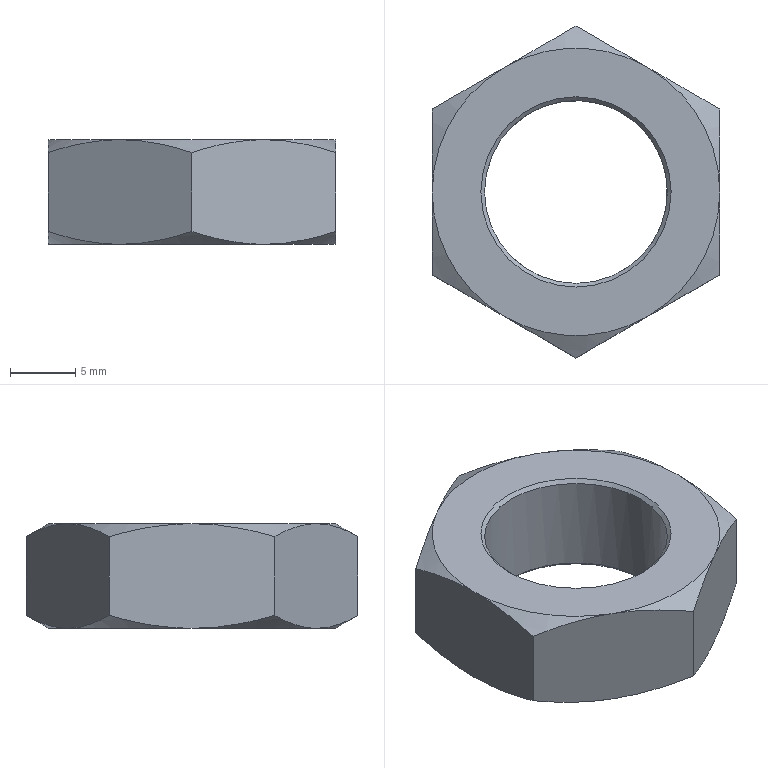Part | NX | features CDQ2B32-35DM_RodEndNuts_M14X1.5 2 | 1 solid | 23 faces | box 21.997 x 25.4 x 8 mm | volume 2094 mm3 | cone 14 | plane 8 | cylinder 1 | commonest cylinder face diameters 14 x1
STEP:
#1=CARTESIAN_POINT('',(-5.655,-9.435,4.));
#2=VERTEX_POINT('',#1);
#3=CARTESIAN_POINT('',(-10.999,-0.1803,4.));
#4=VERTEX_POINT('',#3);
#5=CARTESIAN_POINT('',(0.,0.,4.));
#6=DIRECTION('',(0.,0.,-1.));
#7=DIRECTION('',(-1.,0.,0.));
#8=AXIS2_PLACEMENT_3D('',#5,#6,#7);
#9=CIRCLE('',#8,11.);
#10=EDGE_CURVE('',#2,#4,#9,.T.);
#11=ORIENTED_EDGE('',*,*,#10,.F.);
#12=CARTESIAN_POINT('',(-5.343,-9.615,4.));
#13=VERTEX_POINT('',#12);
#14=CARTESIAN_POINT('',(-5.655,-9.435,4.));
#15=DIRECTION('',(0.866,-0.5,0.));
#16=VECTOR('',#15,1000.);
#17=LINE('',#14,#16);
#18=EDGE_CURVE('',#2,#13,#17,.T.);
#19=ORIENTED_EDGE('',*,*,#18,.T.);
#20=CARTESIAN_POINT('',(5.343,-9.615,4.));
#21=VERTEX_POINT('',#20);
#22=CARTESIAN_POINT('',(0.,0.,4.));
#23=DIRECTION('',(0.,0.,-1.));
#24=DIRECTION('',(-1.,0.,0.));
#25=AXIS2_PLACEMENT_3D('',#22,#23,#24);
#26=CIRCLE('',#25,11.);
#27=EDGE_CURVE('',#21,#13,#26,.T.);
#28=ORIENTED_EDGE('',*,*,#27,.F.);
#29=CARTESIAN_POINT('',(5.655,-9.435,4.));
#30=VERTEX_POINT('',#29);
#31=CARTESIAN_POINT('',(5.343,-9.615,4.));
#32=DIRECTION('',(0.866,0.5,0.));
#33=VECTOR('',#32,1000.);
#34=LINE('',#31,#33);
#35=EDGE_CURVE('',#21,#30,#34,.T.);
#36=ORIENTED_EDGE('',*,*,#35,.T.);
#37=CARTESIAN_POINT('',(10.999,-0.1803,4.));
#38=VERTEX_POINT('',#37);
#39=CARTESIAN_POINT('',(0.,0.,4.));
#40=DIRECTION('',(0.,0.,-1.));
#41=DIRECTION('',(-1.,0.,0.));
#42=AXIS2_PLACEMENT_3D('',#39,#40,#41);
#43=CIRCLE('',#42,11.);
#44=EDGE_CURVE('',#38,#30,#43,.T.);
#45=ORIENTED_EDGE('',*,*,#44,.F.);
#46=CARTESIAN_POINT('',(10.999,0.1803,4.));
#47=VERTEX_POINT('',#46);
#48=CARTESIAN_POINT('',(10.999,7.,4.));
#49=DIRECTION('',(0.,1.,0.));
#50=VECTOR('',#49,1000.);
#51=LINE('',#48,#50);
#52=EDGE_CURVE('',#38,#47,#51,.T.);
#53=ORIENTED_EDGE('',*,*,#52,.T.);
#54=CARTESIAN_POINT('',(5.655,9.435,4.));
#55=VERTEX_POINT('',#54);
#56=CARTESIAN_POINT('',(0.,0.,4.));
#57=DIRECTION('',(0.,0.,-1.));
#58=DIRECTION('',(0.,1.,0.));
#59=AXIS2_PLACEMENT_3D('',#56,#57,#58);
#60=CIRCLE('',#59,11.);
#61=EDGE_CURVE('',#55,#47,#60,.T.);
#62=ORIENTED_EDGE('',*,*,#61,.F.);
#63=CARTESIAN_POINT('',(5.343,9.615,4.));
#64=VERTEX_POINT('',#63);
#65=CARTESIAN_POINT('',(5.655,9.435,4.));
#66=DIRECTION('',(-0.866,0.5,0.));
#67=VECTOR('',#66,1000.);
#68=LINE('',#65,#67);
#69=EDGE_CURVE('',#55,#64,#68,.T.);
#70=ORIENTED_EDGE('',*,*,#69,.T.);
#71=CARTESIAN_POINT('',(-5.343,9.615,4.));
#72=VERTEX_POINT('',#71);
#73=CARTESIAN_POINT('',(0.,0.,4.));
#74=DIRECTION('',(0.,0.,-1.));
#75=DIRECTION('',(0.,1.,0.));
#76=AXIS2_PLACEMENT_3D('',#73,#74,#75);
#77=CIRCLE('',#76,11.);
#78=EDGE_CURVE('',#72,#64,#77,.T.);
#79=ORIENTED_EDGE('',*,*,#78,.F.);
#80=CARTESIAN_POINT('',(-5.655,9.435,4.));
#81=VERTEX_POINT('',#80);
#82=CARTESIAN_POINT('',(-5.343,9.615,4.));
#83=DIRECTION('',(-0.866,-0.5,0.));
#84=VECTOR('',#83,1000.);
#85=LINE('',#82,#84);
#86=EDGE_CURVE('',#72,#81,#85,.T.);
#87=ORIENTED_EDGE('',*,*,#86,.T.);
#88=CARTESIAN_POINT('',(-10.999,0.1803,4.));
#89=VERTEX_POINT('',#88);
#90=CARTESIAN_POINT('',(0.,0.,4.));
#91=DIRECTION('',(0.,0.,-1.));
#92=DIRECTION('',(0.,1.,0.));
#93=AXIS2_PLACEMENT_3D('',#90,#91,#92);
#94=CIRCLE('',#93,11.);
#95=EDGE_CURVE('',#89,#81,#94,.T.);
#96=ORIENTED_EDGE('',*,*,#95,.F.);
#97=CARTESIAN_POINT('',(-10.999,7.,4.));
#98=DIRECTION('',(0.,1.,0.));
#99=VECTOR('',#98,1000.);
#100=LINE('',#97,#99);
#101=EDGE_CURVE('',#89,#4,#100,.F.);
#102=ORIENTED_EDGE('',*,*,#101,.T.);
#103=EDGE_LOOP('',(#11,#19,#28,#36,#45,#53,#62,#70,#79,#87,#96,#102));
#104=FACE_BOUND('',#103,.T.);
#105=CARTESIAN_POINT('',(7.28,0.,4.));
#106=VERTEX_POINT('',#105);
#107=CARTESIAN_POINT('',(0.,0.,4.));
#108=DIRECTION('',(0.,0.,1.));
#109=DIRECTION('',(1.,0.,0.));
#110=AXIS2_PLACEMENT_3D('',#107,#108,#109);
#111=CIRCLE('',#110,7.28);
#112=EDGE_CURVE('',#106,#106,#111,.F.);
#113=ORIENTED_EDGE('',*,*,#112,.T.);
#114=EDGE_LOOP('',(#113));
#115=FACE_BOUND('',#114,.T.);
#116=CARTESIAN_POINT('',(0.,7.,4.));
#117=DIRECTION('',(0.,0.,1.));
#118=DIRECTION('',(1.,0.,0.));
#119=AXIS2_PLACEMENT_3D('',#116,#117,#118);
#120=PLANE('',#119);
#121=ADVANCED_FACE('',(#104,#115),#120,.T.);
#122=CARTESIAN_POINT('',(-7.,0.,3.72));
#123=VERTEX_POINT('',#122);
#124=CARTESIAN_POINT('',(0.,0.,3.72));
#125=DIRECTION('',(0.,0.,-1.));
#126=DIRECTION('',(-1.,0.,0.));
#127=AXIS2_PLACEMENT_3D('',#124,#125,#126);
#128=CIRCLE('',#127,7.);
#129=EDGE_CURVE('',#123,#123,#128,.T.);
#130=ORIENTED_EDGE('',*,*,#129,.T.);
#131=EDGE_LOOP('',(#130));
#132=FACE_BOUND('',#131,.T.);
#133=ORIENTED_EDGE('',*,*,#112,.F.);
#134=EDGE_LOOP('',(#133));
#135=FACE_BOUND('',#134,.T.);
#136=CARTESIAN_POINT('',(0.,0.,4.));
#137=DIRECTION('',(0.,0.,1.));
#138=DIRECTION('',(1.,0.,0.));
#139=AXIS2_PLACEMENT_3D('',#136,#137,#138);
#140=CONICAL_SURFACE('',#139,7.28,0.7854);
#141=ADVANCED_FACE('',(#132,#135),#140,.F.);
#142=CARTESIAN_POINT('',(0.,-12.7,3.019));
#143=VERTEX_POINT('',#142);
#144=CARTESIAN_POINT('',(5.343,-9.615,4.));
#145=CARTESIAN_POINT('',(3.52,-10.668,3.98));
#146=CARTESIAN_POINT('',(1.746,-11.692,3.6));
#147=CARTESIAN_POINT('',(0.,-12.7,3.019));
#148=B_SPLINE_CURVE_WITH_KNOTS('',3,(#144,#145,#146,#147),.UNSPECIFIED.,.F.,.F.,(4,4),(0.,0.006247),.UNSPECIFIED.);
#149=EDGE_CURVE('',#21,#143,#148,.T.);
#150=ORIENTED_EDGE('',*,*,#149,.F.);
#151=ORIENTED_EDGE('',*,*,#27,.T.);
#152=CARTESIAN_POINT('',(0.,-12.7,3.019));
#153=CARTESIAN_POINT('',(-1.746,-11.692,3.6));
#154=CARTESIAN_POINT('',(-3.52,-10.668,3.98));
#155=CARTESIAN_POINT('',(-5.343,-9.615,4.));
#156=B_SPLINE_CURVE_WITH_KNOTS('',3,(#152,#153,#154,#155),.UNSPECIFIED.,.F.,.F.,(4,4),(0.,0.006247),.UNSPECIFIED.);
#157=EDGE_CURVE('',#143,#13,#156,.T.);
#158=ORIENTED_EDGE('',*,*,#157,.F.);
#159=EDGE_LOOP('',(#150,#151,#158));
#160=FACE_BOUND('',#159,.T.);
#161=CARTESIAN_POINT('',(0.,0.,3.013));
#162=DIRECTION('',(0.,0.,-1.));
#163=DIRECTION('',(-1.,0.,0.));
#164=AXIS2_PLACEMENT_3D('',#161,#162,#163);
#165=CONICAL_SURFACE('',#164,12.71,1.047);
#166=ADVANCED_FACE('',(#160),#165,.T.);
#167=CARTESIAN_POINT('',(-10.999,-6.35,3.019));
#168=VERTEX_POINT('',#167);
#169=CARTESIAN_POINT('',(-5.655,-9.435,4.));
#170=CARTESIAN_POINT('',(-7.479,-8.382,3.98));
#171=CARTESIAN_POINT('',(-9.253,-7.358,3.6));
#172=CARTESIAN_POINT('',(-10.999,-6.35,3.019));
#173=B_SPLINE_CURVE_WITH_KNOTS('',3,(#169,#170,#171,#172),.UNSPECIFIED.,.F.,.F.,(4,4),(0.,0.006247),.UNSPECIFIED.);
#174=EDGE_CURVE('',#2,#168,#173,.T.);
#175=ORIENTED_EDGE('',*,*,#174,.F.);
#176=ORIENTED_EDGE('',*,*,#10,.T.);
#177=CARTESIAN_POINT('',(-10.999,-6.35,3.019));
#178=CARTESIAN_POINT('',(-10.999,-4.334,3.6));
#179=CARTESIAN_POINT('',(-10.999,-2.286,3.98));
#180=CARTESIAN_POINT('',(-10.999,-0.1803,4.));
#181=B_SPLINE_CURVE_WITH_KNOTS('',3,(#177,#178,#179,#180),.UNSPECIFIED.,.F.,.F.,(4,4),(0.,0.006247),.UNSPECIFIED.);
#182=EDGE_CURVE('',#168,#4,#181,.T.);
#183=ORIENTED_EDGE('',*,*,#182,.F.);
#184=EDGE_LOOP('',(#175,#176,#183));
#185=FACE_BOUND('',#184,.T.);
#186=CARTESIAN_POINT('',(0.,0.,3.013));
#187=DIRECTION('',(0.,0.,-1.));
#188=DIRECTION('',(-1.,0.,0.));
#189=AXIS2_PLACEMENT_3D('',#186,#187,#188);
#190=CONICAL_SURFACE('',#189,12.71,1.047);
#191=ADVANCED_FACE('',(#185),#190,.T.);
#192=CARTESIAN_POINT('',(-10.999,6.35,3.019));
#193=VERTEX_POINT('',#192);
#194=CARTESIAN_POINT('',(-10.999,0.1803,4.));
#195=CARTESIAN_POINT('',(-10.999,2.286,3.98));
#196=CARTESIAN_POINT('',(-10.999,4.334,3.6));
#197=CARTESIAN_POINT('',(-10.999,6.35,3.019));
#198=B_SPLINE_CURVE_WITH_KNOTS('',3,(#194,#195,#196,#197),.UNSPECIFIED.,.F.,.F.,(4,4),(0.,0.006247),.UNSPECIFIED.);
#199=EDGE_CURVE('',#89,#193,#198,.T.);
#200=ORIENTED_EDGE('',*,*,#199,.F.);
#201=ORIENTED_EDGE('',*,*,#95,.T.);
#202=CARTESIAN_POINT('',(-10.999,6.35,3.019));
#203=CARTESIAN_POINT('',(-9.253,7.358,3.6));
#204=CARTESIAN_POINT('',(-7.479,8.382,3.98));
#205=CARTESIAN_POINT('',(-5.655,9.435,4.));
#206=B_SPLINE_CURVE_WITH_KNOTS('',3,(#202,#203,#204,#205),.UNSPECIFIED.,.F.,.F.,(4,4),(0.,0.006247),.UNSPECIFIED.);
#207=EDGE_CURVE('',#193,#81,#206,.T.);
#208=ORIENTED_EDGE('',*,*,#207,.F.);
#209=EDGE_LOOP('',(#200,#201,#208));
#210=FACE_BOUND('',#209,.T.);
#211=CARTESIAN_POINT('',(0.,0.,3.013));
#212=DIRECTION('',(0.,0.,-1.));
#213=DIRECTION('',(0.,1.,0.));
#214=AXIS2_PLACEMENT_3D('',#211,#212,#213);
#215=CONICAL_SURFACE('',#214,12.71,1.047);
#216=ADVANCED_FACE('',(#210),#215,.T.);
#217=CARTESIAN_POINT('',(0.,12.7,3.019));
#218=VERTEX_POINT('',#217);
#219=CARTESIAN_POINT('',(-5.343,9.615,4.));
#220=CARTESIAN_POINT('',(-3.52,10.668,3.98));
#221=CARTESIAN_POINT('',(-1.746,11.692,3.6));
#222=CARTESIAN_POINT('',(0.,12.7,3.019));
#223=B_SPLINE_CURVE_WITH_KNOTS('',3,(#219,#220,#221,#222),.UNSPECIFIED.,.F.,.F.,(4,4),(0.,0.006247),.UNSPECIFIED.);
#224=EDGE_CURVE('',#72,#218,#223,.T.);
#225=ORIENTED_EDGE('',*,*,#224,.F.);
#226=ORIENTED_EDGE('',*,*,#78,.T.);
#227=CARTESIAN_POINT('',(0.,12.7,3.019));
#228=CARTESIAN_POINT('',(1.746,11.692,3.6));
#229=CARTESIAN_POINT('',(3.52,10.668,3.98));
#230=CARTESIAN_POINT('',(5.343,9.615,4.));
#231=B_SPLINE_CURVE_WITH_KNOTS('',3,(#227,#228,#229,#230),.UNSPECIFIED.,.F.,.F.,(4,4),(0.,0.006247),.UNSPECIFIED.);
#232=EDGE_CURVE('',#218,#64,#231,.T.);
#233=ORIENTED_EDGE('',*,*,#232,.F.);
#234=EDGE_LOOP('',(#225,#226,#233));
#235=FACE_BOUND('',#234,.T.);
#236=CARTESIAN_POINT('',(0.,0.,3.013));
#237=DIRECTION('',(0.,0.,-1.));
#238=DIRECTION('',(0.,1.,0.));
#239=AXIS2_PLACEMENT_3D('',#236,#237,#238);
#240=CONICAL_SURFACE('',#239,12.71,1.047);
#241=ADVANCED_FACE('',(#235),#240,.T.);
#242=CARTESIAN_POINT('',(10.999,6.35,3.019));
#243=VERTEX_POINT('',#242);
#244=CARTESIAN_POINT('',(5.655,9.435,4.));
#245=CARTESIAN_POINT('',(7.479,8.382,3.98));
#246=CARTESIAN_POINT('',(9.253,7.358,3.6));
#247=CARTESIAN_POINT('',(10.999,6.35,3.019));
#248=B_SPLINE_CURVE_WITH_KNOTS('',3,(#244,#245,#246,#247),.UNSPECIFIED.,.F.,.F.,(4,4),(0.,0.006247),.UNSPECIFIED.);
#249=EDGE_CURVE('',#55,#243,#248,.T.);
#250=ORIENTED_EDGE('',*,*,#249,.F.);
#251=ORIENTED_EDGE('',*,*,#61,.T.);
#252=CARTESIAN_POINT('',(10.999,6.35,3.019));
#253=CARTESIAN_POINT('',(10.999,4.334,3.6));
#254=CARTESIAN_POINT('',(10.999,2.286,3.98));
#255=CARTESIAN_POINT('',(10.999,0.1803,4.));
#256=B_SPLINE_CURVE_WITH_KNOTS('',3,(#252,#253,#254,#255),.UNSPECIFIED.,.F.,.F.,(4,4),(0.,0.006247),.UNSPECIFIED.);
#257=EDGE_CURVE('',#243,#47,#256,.T.);
#258=ORIENTED_EDGE('',*,*,#257,.F.);
#259=EDGE_LOOP('',(#250,#251,#258));
#260=FACE_BOUND('',#259,.T.);
#261=CARTESIAN_POINT('',(0.,0.,3.013));
#262=DIRECTION('',(0.,0.,-1.));
#263=DIRECTION('',(0.,1.,0.));
#264=AXIS2_PLACEMENT_3D('',#261,#262,#263);
#265=CONICAL_SURFACE('',#264,12.71,1.047);
#266=ADVANCED_FACE('',(#260),#265,.T.);
#267=CARTESIAN_POINT('',(10.999,-6.35,3.019));
#268=VERTEX_POINT('',#267);
#269=CARTESIAN_POINT('',(10.999,-6.35,3.019));
#270=CARTESIAN_POINT('',(9.253,-7.358,3.6));
#271=CARTESIAN_POINT('',(7.479,-8.382,3.98));
#272=CARTESIAN_POINT('',(5.655,-9.435,4.));
#273=B_SPLINE_CURVE_WITH_KNOTS('',3,(#269,#270,#271,#272),.UNSPECIFIED.,.F.,.F.,(4,4),(0.,0.006247),.UNSPECIFIED.);
#274=EDGE_CURVE('',#268,#30,#273,.T.);
#275=ORIENTED_EDGE('',*,*,#274,.F.);
#276=CARTESIAN_POINT('',(10.999,-0.1803,4.));
#277=CARTESIAN_POINT('',(10.999,-2.286,3.98));
#278=CARTESIAN_POINT('',(10.999,-4.334,3.6));
#279=CARTESIAN_POINT('',(10.999,-6.35,3.019));
#280=B_SPLINE_CURVE_WITH_KNOTS('',3,(#276,#277,#278,#279),.UNSPECIFIED.,.F.,.F.,(4,4),(0.,0.006247),.UNSPECIFIED.);
#281=EDGE_CURVE('',#38,#268,#280,.T.);
#282=ORIENTED_EDGE('',*,*,#281,.F.);
#283=ORIENTED_EDGE('',*,*,#44,.T.);
#284=EDGE_LOOP('',(#275,#282,#283));
#285=FACE_BOUND('',#284,.T.);
#286=CARTESIAN_POINT('',(0.,0.,3.013));
#287=DIRECTION('',(0.,0.,-1.));
#288=DIRECTION('',(-1.,0.,0.));
#289=AXIS2_PLACEMENT_3D('',#286,#287,#288);
#290=CONICAL_SURFACE('',#289,12.71,1.047);
#291=ADVANCED_FACE('',(#285),#290,.T.);
#292=ORIENTED_EDGE('',*,*,#129,.F.);
#293=EDGE_LOOP('',(#292));
#294=FACE_BOUND('',#293,.T.);
#295=CARTESIAN_POINT('',(-7.,0.,-3.72));
#296=VERTEX_POINT('',#295);
#297=CARTESIAN_POINT('',(0.,0.,-3.72));
#298=DIRECTION('',(0.,0.,-1.));
#299=DIRECTION('',(-1.,0.,0.));
#300=AXIS2_PLACEMENT_3D('',#297,#298,#299);
#301=CIRCLE('',#300,7.);
#302=EDGE_CURVE('',#296,#296,#301,.T.);
#303=ORIENTED_EDGE('',*,*,#302,.T.);
#304=EDGE_LOOP('',(#303));
#305=FACE_BOUND('',#304,.T.);
#306=CARTESIAN_POINT('',(0.,0.,27.389));
#307=DIRECTION('',(0.,0.,-1.));
#308=DIRECTION('',(-1.,0.,0.));
#309=AXIS2_PLACEMENT_3D('',#306,#307,#308);
#310=CYLINDRICAL_SURFACE('',#309,7.);
#311=ADVANCED_FACE('',(#294,#305),#310,.F.);
#312=CARTESIAN_POINT('',(5.343,-9.615,-4.));
#313=VERTEX_POINT('',#312);
#314=CARTESIAN_POINT('',(5.655,-9.435,-4.));
#315=VERTEX_POINT('',#314);
#316=CARTESIAN_POINT('',(0.,-12.7,-4.));
#317=DIRECTION('',(0.866,0.5,0.));
#318=VECTOR('',#317,1000.);
#319=LINE('',#316,#318);
#320=EDGE_CURVE('',#313,#315,#319,.T.);
#321=ORIENTED_EDGE('',*,*,#320,.T.);
#322=CARTESIAN_POINT('',(10.999,-6.35,-3.019));
#323=VERTEX_POINT('',#322);
#324=CARTESIAN_POINT('',(10.999,-6.35,-3.019));
#325=CARTESIAN_POINT('',(9.253,-7.358,-3.6));
#326=CARTESIAN_POINT('',(7.479,-8.382,-3.98));
#327=CARTESIAN_POINT('',(5.655,-9.435,-4.));
#328=B_SPLINE_CURVE_WITH_KNOTS('',3,(#324,#325,#326,#327),.UNSPECIFIED.,.F.,.F.,(4,4),(0.,0.006247),.UNSPECIFIED.);
#329=EDGE_CURVE('',#323,#315,#328,.T.);
#330=ORIENTED_EDGE('',*,*,#329,.F.);
#331=CARTESIAN_POINT('',(10.999,-6.35,-4.));
#332=DIRECTION('',(0.,0.,-1.));
#333=VECTOR('',#332,1000.);
#334=LINE('',#331,#333);
#335=EDGE_CURVE('',#268,#323,#334,.T.);
#336=ORIENTED_EDGE('',*,*,#335,.F.);
#337=ORIENTED_EDGE('',*,*,#274,.T.);
#338=ORIENTED_EDGE('',*,*,#35,.F.);
#339=ORIENTED_EDGE('',*,*,#149,.T.);
#340=CARTESIAN_POINT('',(-0.000000012,-12.7,-3.019));
#341=VERTEX_POINT('',#340);
#342=CARTESIAN_POINT('',(0.,-12.7,-4.));
#343=DIRECTION('',(0.,0.,1.));
#344=VECTOR('',#343,1000.);
#345=LINE('',#342,#344);
#346=EDGE_CURVE('',#341,#143,#345,.T.);
#347=ORIENTED_EDGE('',*,*,#346,.F.);
#348=CARTESIAN_POINT('',(5.343,-9.615,-4.));
#349=CARTESIAN_POINT('',(3.52,-10.668,-3.98));
#350=CARTESIAN_POINT('',(1.746,-11.692,-3.6));
#351=CARTESIAN_POINT('',(0.000000023,-12.7,-3.019));
#352=B_SPLINE_CURVE_WITH_KNOTS('',3,(#348,#349,#350,#351),.UNSPECIFIED.,.F.,.F.,(4,4),(0.,0.006247),.UNSPECIFIED.);
#353=EDGE_CURVE('',#313,#341,#352,.T.);
#354=ORIENTED_EDGE('',*,*,#353,.F.);
#355=EDGE_LOOP('',(#321,#330,#336,#337,#338,#339,#347,#354));
#356=FACE_BOUND('',#355,.T.);
#357=CARTESIAN_POINT('',(0.,-12.7,-4.));
#358=DIRECTION('',(0.5,-0.866,0.));
#359=DIRECTION('',(0.866,0.5,0.));
#360=AXIS2_PLACEMENT_3D('',#357,#358,#359);
#361=PLANE('',#360);
#362=ADVANCED_FACE('',(#356),#361,.T.);
#363=CARTESIAN_POINT('',(-5.655,-9.435,-4.));
#364=VERTEX_POINT('',#363);
#365=CARTESIAN_POINT('',(-5.343,-9.615,-4.));
#366=VERTEX_POINT('',#365);
#367=CARTESIAN_POINT('',(-10.999,-6.35,-4.));
#368=DIRECTION('',(0.866,-0.5,0.));
#369=VECTOR('',#368,1000.);
#370=LINE('',#367,#369);
#371=EDGE_CURVE('',#364,#366,#370,.T.);
#372=ORIENTED_EDGE('',*,*,#371,.T.);
#373=CARTESIAN_POINT('',(-0.000000023,-12.7,-3.019));
#374=CARTESIAN_POINT('',(-1.746,-11.692,-3.6));
#375=CARTESIAN_POINT('',(-3.52,-10.668,-3.98));
#376=CARTESIAN_POINT('',(-5.343,-9.615,-4.));
#377=B_SPLINE_CURVE_WITH_KNOTS('',3,(#373,#374,#375,#376),.UNSPECIFIED.,.F.,.F.,(4,4),(0.,0.006247),.UNSPECIFIED.);
#378=EDGE_CURVE('',#341,#366,#377,.T.);
#379=ORIENTED_EDGE('',*,*,#378,.F.);
#380=ORIENTED_EDGE('',*,*,#346,.T.);
#381=ORIENTED_EDGE('',*,*,#157,.T.);
#382=ORIENTED_EDGE('',*,*,#18,.F.);
#383=ORIENTED_EDGE('',*,*,#174,.T.);
#384=CARTESIAN_POINT('',(-10.999,-6.35,-3.019));
#385=VERTEX_POINT('',#384);
#386=CARTESIAN_POINT('',(-10.999,-6.35,-4.));
#387=DIRECTION('',(0.,0.,1.));
#388=VECTOR('',#387,1000.);
#389=LINE('',#386,#388);
#390=EDGE_CURVE('',#385,#168,#389,.T.);
#391=ORIENTED_EDGE('',*,*,#390,.F.);
#392=CARTESIAN_POINT('',(-5.655,-9.435,-4.));
#393=CARTESIAN_POINT('',(-7.479,-8.382,-3.98));
#394=CARTESIAN_POINT('',(-9.253,-7.358,-3.6));
#395=CARTESIAN_POINT('',(-10.999,-6.35,-3.019));
#396=B_SPLINE_CURVE_WITH_KNOTS('',3,(#392,#393,#394,#395),.UNSPECIFIED.,.F.,.F.,(4,4),(0.,0.006247),.UNSPECIFIED.);
#397=EDGE_CURVE('',#364,#385,#396,.T.);
#398=ORIENTED_EDGE('',*,*,#397,.F.);
#399=EDGE_LOOP('',(#372,#379,#380,#381,#382,#383,#391,#398));
#400=FACE_BOUND('',#399,.T.);
#401=CARTESIAN_POINT('',(-10.999,-6.35,-4.));
#402=DIRECTION('',(-0.5,-0.866,0.));
#403=DIRECTION('',(0.866,-0.5,0.));
#404=AXIS2_PLACEMENT_3D('',#401,#402,#403);
#405=PLANE('',#404);
#406=ADVANCED_FACE('',(#400),#405,.T.);
#407=CARTESIAN_POINT('',(-10.999,0.1803,-4.));
#408=VERTEX_POINT('',#407);
#409=CARTESIAN_POINT('',(-10.999,-0.1803,-4.));
#410=VERTEX_POINT('',#409);
#411=CARTESIAN_POINT('',(-10.999,6.35,-4.));
#412=DIRECTION('',(0.,1.,0.));
#413=VECTOR('',#412,1000.);
#414=LINE('',#411,#413);
#415=EDGE_CURVE('',#408,#410,#414,.F.);
#416=ORIENTED_EDGE('',*,*,#415,.T.);
#417=CARTESIAN_POINT('',(-10.999,-6.35,-3.019));
#418=CARTESIAN_POINT('',(-10.999,-4.334,-3.6));
#419=CARTESIAN_POINT('',(-10.999,-2.286,-3.98));
#420=CARTESIAN_POINT('',(-10.999,-0.1803,-4.));
#421=B_SPLINE_CURVE_WITH_KNOTS('',3,(#417,#418,#419,#420),.UNSPECIFIED.,.F.,.F.,(4,4),(0.,0.006247),.UNSPECIFIED.);
#422=EDGE_CURVE('',#385,#410,#421,.T.);
#423=ORIENTED_EDGE('',*,*,#422,.F.);
#424=ORIENTED_EDGE('',*,*,#390,.T.);
#425=ORIENTED_EDGE('',*,*,#182,.T.);
#426=ORIENTED_EDGE('',*,*,#101,.F.);
#427=ORIENTED_EDGE('',*,*,#199,.T.);
#428=CARTESIAN_POINT('',(-10.999,6.35,-3.019));
#429=VERTEX_POINT('',#428);
#430=CARTESIAN_POINT('',(-10.999,6.35,-4.));
#431=DIRECTION('',(0.,0.,1.));
#432=VECTOR('',#431,1000.);
#433=LINE('',#430,#432);
#434=EDGE_CURVE('',#429,#193,#433,.T.);
#435=ORIENTED_EDGE('',*,*,#434,.F.);
#436=CARTESIAN_POINT('',(-10.999,0.1803,-4.));
#437=CARTESIAN_POINT('',(-10.999,2.286,-3.98));
#438=CARTESIAN_POINT('',(-10.999,4.334,-3.6));
#439=CARTESIAN_POINT('',(-10.999,6.35,-3.019));
#440=B_SPLINE_CURVE_WITH_KNOTS('',3,(#436,#437,#438,#439),.UNSPECIFIED.,.F.,.F.,(4,4),(0.,0.006247),.UNSPECIFIED.);
#441=EDGE_CURVE('',#408,#429,#440,.T.);
#442=ORIENTED_EDGE('',*,*,#441,.F.);
#443=EDGE_LOOP('',(#416,#423,#424,#425,#426,#427,#435,#442));
#444=FACE_BOUND('',#443,.T.);
#445=CARTESIAN_POINT('',(-10.999,6.35,-4.));
#446=DIRECTION('',(-1.,0.,0.));
#447=DIRECTION('',(0.,0.,1.));
#448=AXIS2_PLACEMENT_3D('',#445,#446,#447);
#449=PLANE('',#448);
#450=ADVANCED_FACE('',(#444),#449,.T.);
#451=CARTESIAN_POINT('',(-5.343,9.615,-4.));
#452=VERTEX_POINT('',#451);
#453=CARTESIAN_POINT('',(-5.655,9.435,-4.));
#454=VERTEX_POINT('',#453);
#455=CARTESIAN_POINT('',(0.,12.7,-4.));
#456=DIRECTION('',(-0.866,-0.5,0.));
#457=VECTOR('',#456,1000.);
#458=LINE('',#455,#457);
#459=EDGE_CURVE('',#452,#454,#458,.T.);
#460=ORIENTED_EDGE('',*,*,#459,.T.);
#461=CARTESIAN_POINT('',(-10.999,6.35,-3.019));
#462=CARTESIAN_POINT('',(-9.253,7.358,-3.6));
#463=CARTESIAN_POINT('',(-7.479,8.382,-3.98));
#464=CARTESIAN_POINT('',(-5.655,9.435,-4.));
#465=B_SPLINE_CURVE_WITH_KNOTS('',3,(#461,#462,#463,#464),.UNSPECIFIED.,.F.,.F.,(4,4),(0.,0.006247),.UNSPECIFIED.);
#466=EDGE_CURVE('',#429,#454,#465,.T.);
#467=ORIENTED_EDGE('',*,*,#466,.F.);
#468=ORIENTED_EDGE('',*,*,#434,.T.);
#469=ORIENTED_EDGE('',*,*,#207,.T.);
#470=ORIENTED_EDGE('',*,*,#86,.F.);
#471=ORIENTED_EDGE('',*,*,#224,.T.);
#472=CARTESIAN_POINT('',(-0.000000014,12.7,-3.019));
#473=VERTEX_POINT('',#472);
#474=CARTESIAN_POINT('',(0.,12.7,-4.));
#475=DIRECTION('',(0.,0.,1.));
#476=VECTOR('',#475,1000.);
#477=LINE('',#474,#476);
#478=EDGE_CURVE('',#473,#218,#477,.T.);
#479=ORIENTED_EDGE('',*,*,#478,.F.);
#480=CARTESIAN_POINT('',(-5.343,9.615,-4.));
#481=CARTESIAN_POINT('',(-3.52,10.668,-3.98));
#482=CARTESIAN_POINT('',(-1.746,11.692,-3.6));
#483=CARTESIAN_POINT('',(-0.000000075,12.7,-3.019));
#484=B_SPLINE_CURVE_WITH_KNOTS('',3,(#480,#481,#482,#483),.UNSPECIFIED.,.F.,.F.,(4,4),(0.,0.006247),.UNSPECIFIED.);
#485=EDGE_CURVE('',#452,#473,#484,.T.);
#486=ORIENTED_EDGE('',*,*,#485,.F.);
#487=EDGE_LOOP('',(#460,#467,#468,#469,#470,#471,#479,#486));
#488=FACE_BOUND('',#487,.T.);
#489=CARTESIAN_POINT('',(0.,12.7,-4.));
#490=DIRECTION('',(-0.5,0.866,0.));
#491=DIRECTION('',(-0.866,-0.5,0.));
#492=AXIS2_PLACEMENT_3D('',#489,#490,#491);
#493=PLANE('',#492);
#494=ADVANCED_FACE('',(#488),#493,.T.);
#495=CARTESIAN_POINT('',(5.655,9.435,-4.));
#496=VERTEX_POINT('',#495);
#497=CARTESIAN_POINT('',(5.343,9.615,-4.));
#498=VERTEX_POINT('',#497);
#499=CARTESIAN_POINT('',(10.999,6.35,-4.));
#500=DIRECTION('',(-0.866,0.5,0.));
#501=VECTOR('',#500,1000.);
#502=LINE('',#499,#501);
#503=EDGE_CURVE('',#496,#498,#502,.T.);
#504=ORIENTED_EDGE('',*,*,#503,.T.);
#505=CARTESIAN_POINT('',(-0.000000029,12.7,-3.019));
#506=CARTESIAN_POINT('',(1.746,11.692,-3.6));
#507=CARTESIAN_POINT('',(3.52,10.668,-3.98));
#508=CARTESIAN_POINT('',(5.343,9.615,-4.));
#509=B_SPLINE_CURVE_WITH_KNOTS('',3,(#505,#506,#507,#508),.UNSPECIFIED.,.F.,.F.,(4,4),(0.,0.006247),.UNSPECIFIED.);
#510=EDGE_CURVE('',#473,#498,#509,.T.);
#511=ORIENTED_EDGE('',*,*,#510,.F.);
#512=ORIENTED_EDGE('',*,*,#478,.T.);
#513=ORIENTED_EDGE('',*,*,#232,.T.);
#514=ORIENTED_EDGE('',*,*,#69,.F.);
#515=ORIENTED_EDGE('',*,*,#249,.T.);
#516=CARTESIAN_POINT('',(10.999,6.35,-3.019));
#517=VERTEX_POINT('',#516);
#518=CARTESIAN_POINT('',(10.999,6.35,-4.));
#519=DIRECTION('',(0.,0.,-1.));
#520=VECTOR('',#519,1000.);
#521=LINE('',#518,#520);
#522=EDGE_CURVE('',#517,#243,#521,.F.);
#523=ORIENTED_EDGE('',*,*,#522,.F.);
#524=CARTESIAN_POINT('',(5.655,9.435,-4.));
#525=CARTESIAN_POINT('',(7.479,8.382,-3.98));
#526=CARTESIAN_POINT('',(9.253,7.358,-3.6));
#527=CARTESIAN_POINT('',(10.999,6.35,-3.019));
#528=B_SPLINE_CURVE_WITH_KNOTS('',3,(#524,#525,#526,#527),.UNSPECIFIED.,.F.,.F.,(4,4),(0.,0.006247),.UNSPECIFIED.);
#529=EDGE_CURVE('',#496,#517,#528,.T.);
#530=ORIENTED_EDGE('',*,*,#529,.F.);
#531=EDGE_LOOP('',(#504,#511,#512,#513,#514,#515,#523,#530));
#532=FACE_BOUND('',#531,.T.);
#533=CARTESIAN_POINT('',(10.999,6.35,-4.));
#534=DIRECTION('',(0.5,0.866,0.));
#535=DIRECTION('',(-0.866,0.5,0.));
#536=AXIS2_PLACEMENT_3D('',#533,#534,#535);
#537=PLANE('',#536);
#538=ADVANCED_FACE('',(#532),#537,.T.);
#539=CARTESIAN_POINT('',(10.999,-0.1803,-4.));
#540=VERTEX_POINT('',#539);
#541=CARTESIAN_POINT('',(10.999,0.1803,-4.));
#542=VERTEX_POINT('',#541);
#543=CARTESIAN_POINT('',(10.999,-6.35,-4.));
#544=DIRECTION('',(0.,1.,0.));
#545=VECTOR('',#544,1000.);
#546=LINE('',#543,#545);
#547=EDGE_CURVE('',#540,#542,#546,.T.);
#548=ORIENTED_EDGE('',*,*,#547,.T.);
#549=CARTESIAN_POINT('',(10.999,6.35,-3.019));
#550=CARTESIAN_POINT('',(10.999,4.334,-3.6));
#551=CARTESIAN_POINT('',(10.999,2.286,-3.98));
#552=CARTESIAN_POINT('',(10.999,0.1803,-4.));
#553=B_SPLINE_CURVE_WITH_KNOTS('',3,(#549,#550,#551,#552),.UNSPECIFIED.,.F.,.F.,(4,4),(0.,0.006247),.UNSPECIFIED.);
#554=EDGE_CURVE('',#517,#542,#553,.T.);
#555=ORIENTED_EDGE('',*,*,#554,.F.);
#556=ORIENTED_EDGE('',*,*,#522,.T.);
#557=ORIENTED_EDGE('',*,*,#257,.T.);
#558=ORIENTED_EDGE('',*,*,#52,.F.);
#559=ORIENTED_EDGE('',*,*,#281,.T.);
#560=ORIENTED_EDGE('',*,*,#335,.T.);
#561=CARTESIAN_POINT('',(10.999,-0.1803,-4.));
#562=CARTESIAN_POINT('',(10.999,-2.286,-3.98));
#563=CARTESIAN_POINT('',(10.999,-4.334,-3.6));
#564=CARTESIAN_POINT('',(10.999,-6.35,-3.019));
#565=B_SPLINE_CURVE_WITH_KNOTS('',3,(#561,#562,#563,#564),.UNSPECIFIED.,.F.,.F.,(4,4),(0.,0.006247),.UNSPECIFIED.);
#566=EDGE_CURVE('',#540,#323,#565,.T.);
#567=ORIENTED_EDGE('',*,*,#566,.F.);
#568=EDGE_LOOP('',(#548,#555,#556,#557,#558,#559,#560,#567));
#569=FACE_BOUND('',#568,.T.);
#570=CARTESIAN_POINT('',(10.999,-6.35,-4.));
#571=DIRECTION('',(1.,0.,0.));
#572=DIRECTION('',(0.,0.,-1.));
#573=AXIS2_PLACEMENT_3D('',#570,#571,#572);
#574=PLANE('',#573);
#575=ADVANCED_FACE('',(#569),#574,.T.);
#576=ORIENTED_EDGE('',*,*,#302,.F.);
#577=EDGE_LOOP('',(#576));
#578=FACE_BOUND('',#577,.T.);
#579=CARTESIAN_POINT('',(-7.28,0.,-4.));
#580=VERTEX_POINT('',#579);
#581=CARTESIAN_POINT('',(0.,0.,-4.));
#582=DIRECTION('',(0.,0.,-1.));
#583=DIRECTION('',(-1.,0.,0.));
#584=AXIS2_PLACEMENT_3D('',#581,#582,#583);
#585=CIRCLE('',#584,7.28);
#586=EDGE_CURVE('',#580,#580,#585,.F.);
#587=ORIENTED_EDGE('',*,*,#586,.F.);
#588=EDGE_LOOP('',(#587));
#589=FACE_BOUND('',#588,.T.);
#590=CARTESIAN_POINT('',(0.,0.,-4.));
#591=DIRECTION('',(0.,0.,-1.));
#592=DIRECTION('',(-1.,0.,0.));
#593=AXIS2_PLACEMENT_3D('',#590,#591,#592);
#594=CONICAL_SURFACE('',#593,7.28,0.7854);
#595=ADVANCED_FACE('',(#578,#589),#594,.F.);
#596=ORIENTED_EDGE('',*,*,#329,.T.);
#597=CARTESIAN_POINT('',(0.,0.,-4.));
#598=DIRECTION('',(0.,0.,1.));
#599=DIRECTION('',(1.,0.,0.));
#600=AXIS2_PLACEMENT_3D('',#597,#598,#599);
#601=CIRCLE('',#600,11.);
#602=EDGE_CURVE('',#540,#315,#601,.F.);
#603=ORIENTED_EDGE('',*,*,#602,.F.);
#604=ORIENTED_EDGE('',*,*,#566,.T.);
#605=EDGE_LOOP('',(#596,#603,#604));
#606=FACE_BOUND('',#605,.T.);
#607=CARTESIAN_POINT('',(0.,0.,-3.013));
#608=DIRECTION('',(0.,0.,1.));
#609=DIRECTION('',(1.,0.,0.));
#610=AXIS2_PLACEMENT_3D('',#607,#608,#609);
#611=CONICAL_SURFACE('',#610,12.71,1.047);
#612=ADVANCED_FACE('',(#606),#611,.T.);
#613=ORIENTED_EDGE('',*,*,#353,.T.);
#614=ORIENTED_EDGE('',*,*,#378,.T.);
#615=CARTESIAN_POINT('',(0.,0.,-4.));
#616=DIRECTION('',(0.,0.,1.));
#617=DIRECTION('',(0.,-1.,0.));
#618=AXIS2_PLACEMENT_3D('',#615,#616,#617);
#619=CIRCLE('',#618,11.);
#620=EDGE_CURVE('',#313,#366,#619,.F.);
#621=ORIENTED_EDGE('',*,*,#620,.F.);
#622=EDGE_LOOP('',(#613,#614,#621));
#623=FACE_BOUND('',#622,.T.);
#624=CARTESIAN_POINT('',(0.,0.,-3.013));
#625=DIRECTION('',(0.,0.,1.));
#626=DIRECTION('',(0.,-1.,0.));
#627=AXIS2_PLACEMENT_3D('',#624,#625,#626);
#628=CONICAL_SURFACE('',#627,12.71,1.047);
#629=ADVANCED_FACE('',(#623),#628,.T.);
#630=ORIENTED_EDGE('',*,*,#397,.T.);
#631=ORIENTED_EDGE('',*,*,#422,.T.);
#632=CARTESIAN_POINT('',(0.,0.,-4.));
#633=DIRECTION('',(0.,0.,1.));
#634=DIRECTION('',(0.,-1.,0.));
#635=AXIS2_PLACEMENT_3D('',#632,#633,#634);
#636=CIRCLE('',#635,11.);
#637=EDGE_CURVE('',#364,#410,#636,.F.);
#638=ORIENTED_EDGE('',*,*,#637,.F.);
#639=EDGE_LOOP('',(#630,#631,#638));
#640=FACE_BOUND('',#639,.T.);
#641=CARTESIAN_POINT('',(0.,0.,-3.013));
#642=DIRECTION('',(0.,0.,1.));
#643=DIRECTION('',(0.,-1.,0.));
#644=AXIS2_PLACEMENT_3D('',#641,#642,#643);
#645=CONICAL_SURFACE('',#644,12.71,1.047);
#646=ADVANCED_FACE('',(#640),#645,.T.);
#647=ORIENTED_EDGE('',*,*,#441,.T.);
#648=ORIENTED_EDGE('',*,*,#466,.T.);
#649=CARTESIAN_POINT('',(0.,0.,-4.));
#650=DIRECTION('',(0.,0.,1.));
#651=DIRECTION('',(1.,0.,0.));
#652=AXIS2_PLACEMENT_3D('',#649,#650,#651);
#653=CIRCLE('',#652,11.);
#654=EDGE_CURVE('',#408,#454,#653,.F.);
#655=ORIENTED_EDGE('',*,*,#654,.F.);
#656=EDGE_LOOP('',(#647,#648,#655));
#657=FACE_BOUND('',#656,.T.);
#658=CARTESIAN_POINT('',(0.,0.,-3.013));
#659=DIRECTION('',(0.,0.,1.));
#660=DIRECTION('',(1.,0.,0.));
#661=AXIS2_PLACEMENT_3D('',#658,#659,#660);
#662=CONICAL_SURFACE('',#661,12.71,1.047);
#663=ADVANCED_FACE('',(#657),#662,.T.);
#664=ORIENTED_EDGE('',*,*,#485,.T.);
#665=ORIENTED_EDGE('',*,*,#510,.T.);
#666=CARTESIAN_POINT('',(0.,0.,-4.));
#667=DIRECTION('',(0.,0.,1.));
#668=DIRECTION('',(1.,0.,0.));
#669=AXIS2_PLACEMENT_3D('',#666,#667,#668);
#670=CIRCLE('',#669,11.);
#671=EDGE_CURVE('',#452,#498,#670,.F.);
#672=ORIENTED_EDGE('',*,*,#671,.F.);
#673=EDGE_LOOP('',(#664,#665,#672));
#674=FACE_BOUND('',#673,.T.);
#675=CARTESIAN_POINT('',(0.,0.,-3.013));
#676=DIRECTION('',(0.,0.,1.));
#677=DIRECTION('',(1.,0.,0.));
#678=AXIS2_PLACEMENT_3D('',#675,#676,#677);
#679=CONICAL_SURFACE('',#678,12.71,1.047);
#680=ADVANCED_FACE('',(#674),#679,.T.);
#681=ORIENTED_EDGE('',*,*,#529,.T.);
#682=ORIENTED_EDGE('',*,*,#554,.T.);
#683=CARTESIAN_POINT('',(0.,0.,-4.));
#684=DIRECTION('',(0.,0.,1.));
#685=DIRECTION('',(0.,-1.,0.));
#686=AXIS2_PLACEMENT_3D('',#683,#684,#685);
#687=CIRCLE('',#686,11.);
#688=EDGE_CURVE('',#496,#542,#687,.F.);
#689=ORIENTED_EDGE('',*,*,#688,.F.);
#690=EDGE_LOOP('',(#681,#682,#689));
#691=FACE_BOUND('',#690,.T.);
#692=CARTESIAN_POINT('',(0.,0.,-3.013));
#693=DIRECTION('',(0.,0.,1.));
#694=DIRECTION('',(0.,-1.,0.));
#695=AXIS2_PLACEMENT_3D('',#692,#693,#694);
#696=CONICAL_SURFACE('',#695,12.71,1.047);
#697=ADVANCED_FACE('',(#691),#696,.T.);
#698=ORIENTED_EDGE('',*,*,#688,.T.);
#699=ORIENTED_EDGE('',*,*,#547,.F.);
#700=ORIENTED_EDGE('',*,*,#602,.T.);
#701=ORIENTED_EDGE('',*,*,#320,.F.);
#702=ORIENTED_EDGE('',*,*,#620,.T.);
#703=ORIENTED_EDGE('',*,*,#371,.F.);
#704=ORIENTED_EDGE('',*,*,#637,.T.);
#705=ORIENTED_EDGE('',*,*,#415,.F.);
#706=ORIENTED_EDGE('',*,*,#654,.T.);
#707=ORIENTED_EDGE('',*,*,#459,.F.);
#708=ORIENTED_EDGE('',*,*,#671,.T.);
#709=ORIENTED_EDGE('',*,*,#503,.F.);
#710=EDGE_LOOP('',(#698,#699,#700,#701,#702,#703,#704,#705,#706,#707,#708,#709));
#711=FACE_BOUND('',#710,.T.);
#712=ORIENTED_EDGE('',*,*,#586,.T.);
#713=EDGE_LOOP('',(#712));
#714=FACE_BOUND('',#713,.T.);
#715=CARTESIAN_POINT('',(0.,7.,-4.));
#716=DIRECTION('',(0.,0.,-1.));
#717=DIRECTION('',(-1.,0.,0.));
#718=AXIS2_PLACEMENT_3D('',#715,#716,#717);
#719=PLANE('',#718);
#720=ADVANCED_FACE('',(#711,#714),#719,.T.);
#721=CLOSED_SHELL('',(#121,#141,#166,#191,#216,#241,#266,#291,#311,#362,#406,#450,#494,#538,#575,#595,#612,#629,#646,#663,#680,#697,#720));
#722=MANIFOLD_SOLID_BREP('',#721);
#723=(LENGTH_UNIT()NAMED_UNIT(*)SI_UNIT(.MILLI.,.METRE.));
#724=UNCERTAINTY_MEASURE_WITH_UNIT(LENGTH_MEASURE(0.0508),#723,'','');
#725=(NAMED_UNIT(*)PLANE_ANGLE_UNIT()SI_UNIT($,.RADIAN.));
#726=(NAMED_UNIT(*)SI_UNIT($,.STERADIAN.)SOLID_ANGLE_UNIT());
#727=(GEOMETRIC_REPRESENTATION_CONTEXT(3)GLOBAL_UNCERTAINTY_ASSIGNED_CONTEXT((#724))GLOBAL_UNIT_ASSIGNED_CONTEXT((#723,#725,#726))REPRESENTATION_CONTEXT('',''));
#728=ADVANCED_BREP_SHAPE_REPRESENTATION('',(#722),#727);